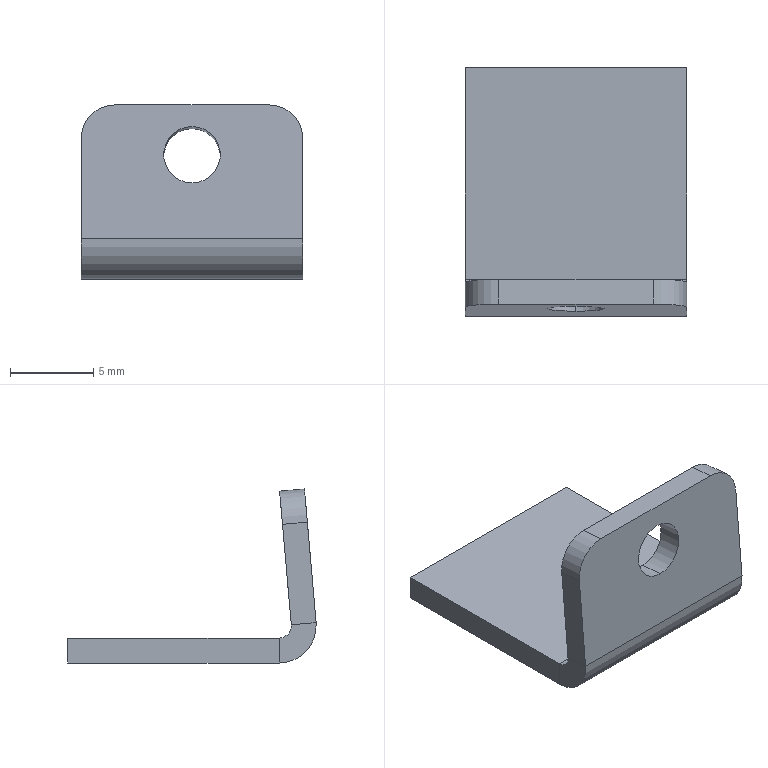Part | STEP file | 07-10 reflector plate (Default) | 1 solid | 18 faces | box 13.3 x 14.933 x 10.46 mm | volume 447.05 mm3 | plane 12 | cylinder 6 | commonest cylinder face diameters 3.4 x2 4 x2 1.473 x1 4.473 x1
STEP:
#1=CARTESIAN_POINT('',(0.,-7.585,7.665));
#2=VERTEX_POINT('',#1);
#3=CARTESIAN_POINT('',(0.,-7.881,4.278));
#4=VERTEX_POINT('',#3);
#5=CARTESIAN_POINT('',(0.,-7.733,5.971));
#6=DIRECTION('',(0.,-0.9962,0.08716));
#7=DIRECTION('',(0.,-0.08716,-0.9962));
#8=AXIS2_PLACEMENT_3D('',#5,#6,#7);
#9=CIRCLE('',#8,1.7);
#10=EDGE_CURVE('',#2,#4,#9,.T.);
#11=ORIENTED_EDGE('',*,*,#10,.T.);
#12=CARTESIAN_POINT('',(0.,-6.387,4.147));
#13=VERTEX_POINT('',#12);
#14=CARTESIAN_POINT('',(0.,-16.349,5.019));
#15=DIRECTION('',(0.,0.9962,-0.08716));
#16=VECTOR('',#15,1000.);
#17=LINE('',#14,#16);
#18=EDGE_CURVE('',#4,#13,#17,.T.);
#19=ORIENTED_EDGE('',*,*,#18,.T.);
#20=CARTESIAN_POINT('',(0.,-6.091,7.534));
#21=VERTEX_POINT('',#20);
#22=CARTESIAN_POINT('',(0.,-6.239,5.841));
#23=DIRECTION('',(0.,0.9962,-0.08716));
#24=DIRECTION('',(0.,0.08716,0.9962));
#25=AXIS2_PLACEMENT_3D('',#22,#23,#24);
#26=CIRCLE('',#25,1.7);
#27=EDGE_CURVE('',#13,#21,#26,.T.);
#28=ORIENTED_EDGE('',*,*,#27,.T.);
#29=CARTESIAN_POINT('',(0.,-16.053,8.406));
#30=DIRECTION('',(0.,0.9962,-0.08716));
#31=VECTOR('',#30,1000.);
#32=LINE('',#29,#31);
#33=EDGE_CURVE('',#2,#21,#32,.T.);
#34=ORIENTED_EDGE('',*,*,#33,.F.);
#35=EDGE_LOOP('',(#11,#19,#28,#34));
#36=FACE_OUTER_BOUND('',#35,.T.);
#37=CARTESIAN_POINT('',(0.,-16.201,6.712));
#38=DIRECTION('',(0.,0.9962,-0.08716));
#39=DIRECTION('',(0.,0.08716,0.9962));
#40=AXIS2_PLACEMENT_3D('',#37,#38,#39);
#41=CYLINDRICAL_SURFACE('',#40,1.7);
#42=ADVANCED_FACE('',(#36),#41,.F.);
#43=CARTESIAN_POINT('',(6.65,-5.946,0.));
#44=VERTEX_POINT('',#43);
#45=CARTESIAN_POINT('',(6.65,6.75,0.));
#46=VERTEX_POINT('',#45);
#47=CARTESIAN_POINT('',(6.65,6.75,0.));
#48=DIRECTION('',(0.,1.,0.));
#49=VECTOR('',#48,1000.);
#50=LINE('',#47,#49);
#51=EDGE_CURVE('',#44,#46,#50,.T.);
#52=ORIENTED_EDGE('',*,*,#51,.F.);
#53=CARTESIAN_POINT('',(6.65,-5.946,-1.5));
#54=VERTEX_POINT('',#53);
#55=CARTESIAN_POINT('',(6.65,-5.946,0.));
#56=DIRECTION('',(0.,0.,-1.));
#57=VECTOR('',#56,1000.);
#58=LINE('',#55,#57);
#59=EDGE_CURVE('',#44,#54,#58,.T.);
#60=ORIENTED_EDGE('',*,*,#59,.T.);
#61=CARTESIAN_POINT('',(6.65,6.75,-1.5));
#62=VERTEX_POINT('',#61);
#63=CARTESIAN_POINT('',(6.65,6.75,-1.5));
#64=DIRECTION('',(0.,1.,0.));
#65=VECTOR('',#64,1000.);
#66=LINE('',#63,#65);
#67=EDGE_CURVE('',#54,#62,#66,.T.);
#68=ORIENTED_EDGE('',*,*,#67,.T.);
#69=CARTESIAN_POINT('',(6.65,6.75,-1.5));
#70=DIRECTION('',(0.,0.,1.));
#71=VECTOR('',#70,1000.);
#72=LINE('',#69,#71);
#73=EDGE_CURVE('',#62,#46,#72,.T.);
#74=ORIENTED_EDGE('',*,*,#73,.T.);
#75=EDGE_LOOP('',(#52,#60,#68,#74));
#76=FACE_OUTER_BOUND('',#75,.T.);
#77=CARTESIAN_POINT('',(6.65,6.75,-1.5));
#78=DIRECTION('',(1.,0.,0.));
#79=DIRECTION('',(0.,1.,0.));
#80=AXIS2_PLACEMENT_3D('',#77,#78,#79);
#81=PLANE('',#80);
#82=ADVANCED_FACE('',(#76),#81,.T.);
#83=CARTESIAN_POINT('',(-6.65,-5.946,-1.5));
#84=VERTEX_POINT('',#83);
#85=CARTESIAN_POINT('',(6.65,-5.946,-1.5));
#86=DIRECTION('',(-1.,0.,0.));
#87=VECTOR('',#86,1000.);
#88=LINE('',#85,#87);
#89=EDGE_CURVE('',#54,#84,#88,.T.);
#90=ORIENTED_EDGE('',*,*,#89,.T.);
#91=CARTESIAN_POINT('',(-6.65,6.75,-1.5));
#92=VERTEX_POINT('',#91);
#93=CARTESIAN_POINT('',(-6.65,6.75,-1.5));
#94=DIRECTION('',(0.,-1.,0.));
#95=VECTOR('',#94,1000.);
#96=LINE('',#93,#95);
#97=EDGE_CURVE('',#92,#84,#96,.T.);
#98=ORIENTED_EDGE('',*,*,#97,.F.);
#99=CARTESIAN_POINT('',(-6.65,6.75,-1.5));
#100=DIRECTION('',(-1.,0.,0.));
#101=VECTOR('',#100,1000.);
#102=LINE('',#99,#101);
#103=EDGE_CURVE('',#62,#92,#102,.T.);
#104=ORIENTED_EDGE('',*,*,#103,.F.);
#105=ORIENTED_EDGE('',*,*,#67,.F.);
#106=EDGE_LOOP('',(#90,#98,#104,#105));
#107=FACE_OUTER_BOUND('',#106,.T.);
#108=CARTESIAN_POINT('',(6.65,-6.75,-1.5));
#109=DIRECTION('',(0.,0.,1.));
#110=DIRECTION('',(1.,0.,0.));
#111=AXIS2_PLACEMENT_3D('',#108,#109,#110);
#112=PLANE('',#111);
#113=ADVANCED_FACE('',(#107),#112,.F.);
#114=CARTESIAN_POINT('',(-6.65,6.75,0.));
#115=VERTEX_POINT('',#114);
#116=CARTESIAN_POINT('',(-6.65,-5.946,0.));
#117=VERTEX_POINT('',#116);
#118=CARTESIAN_POINT('',(-6.65,6.75,0.));
#119=DIRECTION('',(0.,-1.,0.));
#120=VECTOR('',#119,1000.);
#121=LINE('',#118,#120);
#122=EDGE_CURVE('',#115,#117,#121,.T.);
#123=ORIENTED_EDGE('',*,*,#122,.T.);
#124=CARTESIAN_POINT('',(6.65,-5.946,0.));
#125=DIRECTION('',(-1.,0.,0.));
#126=VECTOR('',#125,1000.);
#127=LINE('',#124,#126);
#128=EDGE_CURVE('',#44,#117,#127,.T.);
#129=ORIENTED_EDGE('',*,*,#128,.F.);
#130=ORIENTED_EDGE('',*,*,#51,.T.);
#131=CARTESIAN_POINT('',(-6.65,6.75,0.));
#132=DIRECTION('',(-1.,0.,0.));
#133=VECTOR('',#132,1000.);
#134=LINE('',#131,#133);
#135=EDGE_CURVE('',#46,#115,#134,.T.);
#136=ORIENTED_EDGE('',*,*,#135,.T.);
#137=EDGE_LOOP('',(#123,#129,#130,#136));
#138=FACE_OUTER_BOUND('',#137,.T.);
#139=CARTESIAN_POINT('',(6.65,-6.75,0.));
#140=DIRECTION('',(0.,0.,1.));
#141=DIRECTION('',(1.,0.,0.));
#142=AXIS2_PLACEMENT_3D('',#139,#140,#141);
#143=PLANE('',#142);
#144=ADVANCED_FACE('',(#138),#143,.T.);
#145=CARTESIAN_POINT('',(-6.65,-5.946,0.));
#146=DIRECTION('',(0.,0.,-1.));
#147=VECTOR('',#146,1000.);
#148=LINE('',#145,#147);
#149=EDGE_CURVE('',#117,#84,#148,.T.);
#150=ORIENTED_EDGE('',*,*,#149,.F.);
#151=ORIENTED_EDGE('',*,*,#122,.F.);
#152=CARTESIAN_POINT('',(-6.65,6.75,-1.5));
#153=DIRECTION('',(0.,0.,1.));
#154=VECTOR('',#153,1000.);
#155=LINE('',#152,#154);
#156=EDGE_CURVE('',#92,#115,#155,.T.);
#157=ORIENTED_EDGE('',*,*,#156,.F.);
#158=ORIENTED_EDGE('',*,*,#97,.T.);
#159=EDGE_LOOP('',(#150,#151,#157,#158));
#160=FACE_OUTER_BOUND('',#159,.T.);
#161=CARTESIAN_POINT('',(-6.65,6.75,-1.5));
#162=DIRECTION('',(-1.,0.,0.));
#163=DIRECTION('',(0.,-1.,0.));
#164=AXIS2_PLACEMENT_3D('',#161,#162,#163);
#165=PLANE('',#164);
#166=ADVANCED_FACE('',(#160),#165,.T.);
#167=ORIENTED_EDGE('',*,*,#135,.F.);
#168=ORIENTED_EDGE('',*,*,#73,.F.);
#169=ORIENTED_EDGE('',*,*,#103,.T.);
#170=ORIENTED_EDGE('',*,*,#156,.T.);
#171=EDGE_LOOP('',(#167,#168,#169,#170));
#172=FACE_OUTER_BOUND('',#171,.T.);
#173=CARTESIAN_POINT('',(-6.65,6.75,-1.5));
#174=DIRECTION('',(0.,1.,0.));
#175=DIRECTION('',(0.,0.,1.));
#176=AXIS2_PLACEMENT_3D('',#173,#174,#175);
#177=PLANE('',#176);
#178=ADVANCED_FACE('',(#172),#177,.T.);
#179=CARTESIAN_POINT('',(-6.65,-6.68,0.8008));
#180=VERTEX_POINT('',#179);
#181=CARTESIAN_POINT('',(-6.65,-8.174,0.9315));
#182=VERTEX_POINT('',#181);
#183=CARTESIAN_POINT('',(-6.65,-6.68,0.8008));
#184=DIRECTION('',(0.,-0.9962,0.08716));
#185=VECTOR('',#184,1000.);
#186=LINE('',#183,#185);
#187=EDGE_CURVE('',#180,#182,#186,.T.);
#188=ORIENTED_EDGE('',*,*,#187,.F.);
#189=CARTESIAN_POINT('',(-6.65,-5.946,0.7366));
#190=DIRECTION('',(-1.,0.,0.));
#191=DIRECTION('',(0.,0.,-1.));
#192=AXIS2_PLACEMENT_3D('',#189,#190,#191);
#193=CIRCLE('',#192,0.7366);
#194=EDGE_CURVE('',#117,#180,#193,.T.);
#195=ORIENTED_EDGE('',*,*,#194,.F.);
#196=ORIENTED_EDGE('',*,*,#149,.T.);
#197=CARTESIAN_POINT('',(-6.65,-5.946,0.7366));
#198=DIRECTION('',(-1.,0.,0.));
#199=DIRECTION('',(0.,0.,-1.));
#200=AXIS2_PLACEMENT_3D('',#197,#198,#199);
#201=CIRCLE('',#200,2.237);
#202=EDGE_CURVE('',#84,#182,#201,.T.);
#203=ORIENTED_EDGE('',*,*,#202,.T.);
#204=EDGE_LOOP('',(#188,#195,#196,#203));
#205=FACE_OUTER_BOUND('',#204,.T.);
#206=CARTESIAN_POINT('',(-6.65,-5.946,0.7366));
#207=DIRECTION('',(-1.,0.,0.));
#208=DIRECTION('',(0.,0.,1.));
#209=AXIS2_PLACEMENT_3D('',#206,#207,#208);
#210=PLANE('',#209);
#211=ADVANCED_FACE('',(#205),#210,.T.);
#212=CARTESIAN_POINT('',(6.65,-6.68,0.8008));
#213=VERTEX_POINT('',#212);
#214=CARTESIAN_POINT('',(6.65,-5.946,0.7366));
#215=DIRECTION('',(1.,0.,0.));
#216=DIRECTION('',(0.,0.,-1.));
#217=AXIS2_PLACEMENT_3D('',#214,#215,#216);
#218=CIRCLE('',#217,0.7366);
#219=EDGE_CURVE('',#213,#44,#218,.T.);
#220=ORIENTED_EDGE('',*,*,#219,.F.);
#221=CARTESIAN_POINT('',(6.65,-8.174,0.9315));
#222=VERTEX_POINT('',#221);
#223=CARTESIAN_POINT('',(6.65,-6.68,0.8008));
#224=DIRECTION('',(0.,-0.9962,0.08716));
#225=VECTOR('',#224,1000.);
#226=LINE('',#223,#225);
#227=EDGE_CURVE('',#213,#222,#226,.T.);
#228=ORIENTED_EDGE('',*,*,#227,.T.);
#229=CARTESIAN_POINT('',(6.65,-5.946,0.7366));
#230=DIRECTION('',(1.,0.,0.));
#231=DIRECTION('',(0.,0.,-1.));
#232=AXIS2_PLACEMENT_3D('',#229,#230,#231);
#233=CIRCLE('',#232,2.237);
#234=EDGE_CURVE('',#222,#54,#233,.T.);
#235=ORIENTED_EDGE('',*,*,#234,.T.);
#236=ORIENTED_EDGE('',*,*,#59,.F.);
#237=EDGE_LOOP('',(#220,#228,#235,#236));
#238=FACE_OUTER_BOUND('',#237,.T.);
#239=CARTESIAN_POINT('',(6.65,-5.946,0.7366));
#240=DIRECTION('',(-1.,0.,0.));
#241=DIRECTION('',(0.,0.,1.));
#242=AXIS2_PLACEMENT_3D('',#239,#240,#241);
#243=PLANE('',#242);
#244=ADVANCED_FACE('',(#238),#243,.F.);
#245=ORIENTED_EDGE('',*,*,#89,.F.);
#246=ORIENTED_EDGE('',*,*,#234,.F.);
#247=CARTESIAN_POINT('',(6.65,-8.174,0.9315));
#248=DIRECTION('',(1.,0.,0.));
#249=VECTOR('',#248,1000.);
#250=LINE('',#247,#249);
#251=EDGE_CURVE('',#182,#222,#250,.T.);
#252=ORIENTED_EDGE('',*,*,#251,.F.);
#253=ORIENTED_EDGE('',*,*,#202,.F.);
#254=EDGE_LOOP('',(#245,#246,#252,#253));
#255=FACE_OUTER_BOUND('',#254,.T.);
#256=CARTESIAN_POINT('',(6.65,-5.946,0.7366));
#257=DIRECTION('',(1.,0.,0.));
#258=DIRECTION('',(0.,-0.9962,0.08716));
#259=AXIS2_PLACEMENT_3D('',#256,#257,#258);
#260=CYLINDRICAL_SURFACE('',#259,2.237);
#261=ADVANCED_FACE('',(#255),#260,.T.);
#262=ORIENTED_EDGE('',*,*,#128,.T.);
#263=ORIENTED_EDGE('',*,*,#194,.T.);
#264=CARTESIAN_POINT('',(-6.65,-6.68,0.8008));
#265=DIRECTION('',(1.,0.,0.));
#266=VECTOR('',#265,1000.);
#267=LINE('',#264,#266);
#268=EDGE_CURVE('',#180,#213,#267,.T.);
#269=ORIENTED_EDGE('',*,*,#268,.T.);
#270=ORIENTED_EDGE('',*,*,#219,.T.);
#271=EDGE_LOOP('',(#262,#263,#269,#270));
#272=FACE_OUTER_BOUND('',#271,.T.);
#273=CARTESIAN_POINT('',(6.65,-5.946,0.7366));
#274=DIRECTION('',(1.,0.,0.));
#275=DIRECTION('',(0.,-0.9962,0.08716));
#276=AXIS2_PLACEMENT_3D('',#273,#274,#275);
#277=CYLINDRICAL_SURFACE('',#276,0.7366);
#278=ADVANCED_FACE('',(#272),#277,.F.);
#279=CARTESIAN_POINT('',(6.65,-6.152,6.837));
#280=VERTEX_POINT('',#279);
#281=CARTESIAN_POINT('',(6.65,-6.75,0.));
#282=DIRECTION('',(0.,-0.08716,-0.9962));
#283=VECTOR('',#282,1000.);
#284=LINE('',#281,#283);
#285=EDGE_CURVE('',#280,#213,#284,.T.);
#286=ORIENTED_EDGE('',*,*,#285,.F.);
#287=CARTESIAN_POINT('',(6.65,-7.646,6.968));
#288=VERTEX_POINT('',#287);
#289=CARTESIAN_POINT('',(6.65,-7.646,6.968));
#290=DIRECTION('',(0.,-0.9962,0.08716));
#291=VECTOR('',#290,1000.);
#292=LINE('',#289,#291);
#293=EDGE_CURVE('',#280,#288,#292,.T.);
#294=ORIENTED_EDGE('',*,*,#293,.T.);
#295=CARTESIAN_POINT('',(6.65,-8.244,0.1307));
#296=DIRECTION('',(0.,-0.08716,-0.9962));
#297=VECTOR('',#296,1000.);
#298=LINE('',#295,#297);
#299=EDGE_CURVE('',#288,#222,#298,.T.);
#300=ORIENTED_EDGE('',*,*,#299,.T.);
#301=ORIENTED_EDGE('',*,*,#227,.F.);
#302=EDGE_LOOP('',(#286,#294,#300,#301));
#303=FACE_OUTER_BOUND('',#302,.T.);
#304=CARTESIAN_POINT('',(6.65,-8.244,0.1307));
#305=DIRECTION('',(1.,0.,0.));
#306=DIRECTION('',(0.,0.,-1.));
#307=AXIS2_PLACEMENT_3D('',#304,#305,#306);
#308=PLANE('',#307);
#309=ADVANCED_FACE('',(#303),#308,.T.);
#310=CARTESIAN_POINT('',(-6.65,-7.646,6.968));
#311=VERTEX_POINT('',#310);
#312=CARTESIAN_POINT('',(-6.65,-7.472,8.96));
#313=DIRECTION('',(0.,0.08716,0.9962));
#314=VECTOR('',#313,1000.);
#315=LINE('',#312,#314);
#316=EDGE_CURVE('',#182,#311,#315,.T.);
#317=ORIENTED_EDGE('',*,*,#316,.T.);
#318=CARTESIAN_POINT('',(-6.65,-6.152,6.837));
#319=VERTEX_POINT('',#318);
#320=CARTESIAN_POINT('',(-6.65,-7.646,6.968));
#321=DIRECTION('',(0.,0.9962,-0.08716));
#322=VECTOR('',#321,1000.);
#323=LINE('',#320,#322);
#324=EDGE_CURVE('',#311,#319,#323,.T.);
#325=ORIENTED_EDGE('',*,*,#324,.T.);
#326=CARTESIAN_POINT('',(-6.65,-5.978,8.829));
#327=DIRECTION('',(0.,0.08716,0.9962));
#328=VECTOR('',#327,1000.);
#329=LINE('',#326,#328);
#330=EDGE_CURVE('',#180,#319,#329,.T.);
#331=ORIENTED_EDGE('',*,*,#330,.F.);
#332=ORIENTED_EDGE('',*,*,#187,.T.);
#333=EDGE_LOOP('',(#317,#325,#331,#332));
#334=FACE_OUTER_BOUND('',#333,.T.);
#335=CARTESIAN_POINT('',(-6.65,-7.472,8.96));
#336=DIRECTION('',(-1.,0.,0.));
#337=DIRECTION('',(0.,0.,1.));
#338=AXIS2_PLACEMENT_3D('',#335,#336,#337);
#339=PLANE('',#338);
#340=ADVANCED_FACE('',(#334),#339,.T.);
#341=ORIENTED_EDGE('',*,*,#10,.F.);
#342=CARTESIAN_POINT('',(0.,-7.733,5.971));
#343=DIRECTION('',(0.,-0.9962,0.08716));
#344=DIRECTION('',(0.,-0.08716,-0.9962));
#345=AXIS2_PLACEMENT_3D('',#342,#343,#344);
#346=CIRCLE('',#345,1.7);
#347=EDGE_CURVE('',#4,#2,#346,.T.);
#348=ORIENTED_EDGE('',*,*,#347,.F.);
#349=EDGE_LOOP('',(#341,#348));
#350=FACE_BOUND('',#349,.T.);
#351=ORIENTED_EDGE('',*,*,#299,.F.);
#352=CARTESIAN_POINT('',(4.65,-7.472,8.96));
#353=VERTEX_POINT('',#352);
#354=CARTESIAN_POINT('',(4.65,-7.646,6.968));
#355=DIRECTION('',(0.,-0.9962,0.08716));
#356=DIRECTION('',(0.,-0.08716,-0.9962));
#357=AXIS2_PLACEMENT_3D('',#354,#355,#356);
#358=CIRCLE('',#357,2.);
#359=EDGE_CURVE('',#288,#353,#358,.T.);
#360=ORIENTED_EDGE('',*,*,#359,.T.);
#361=CARTESIAN_POINT('',(-4.65,-7.472,8.96));
#362=VERTEX_POINT('',#361);
#363=CARTESIAN_POINT('',(6.65,-7.472,8.96));
#364=DIRECTION('',(1.,0.,0.));
#365=VECTOR('',#364,1000.);
#366=LINE('',#363,#365);
#367=EDGE_CURVE('',#362,#353,#366,.T.);
#368=ORIENTED_EDGE('',*,*,#367,.F.);
#369=CARTESIAN_POINT('',(-4.65,-7.646,6.968));
#370=DIRECTION('',(0.,-0.9962,0.08716));
#371=DIRECTION('',(0.,-0.08716,-0.9962));
#372=AXIS2_PLACEMENT_3D('',#369,#370,#371);
#373=CIRCLE('',#372,2.);
#374=EDGE_CURVE('',#362,#311,#373,.T.);
#375=ORIENTED_EDGE('',*,*,#374,.T.);
#376=ORIENTED_EDGE('',*,*,#316,.F.);
#377=ORIENTED_EDGE('',*,*,#251,.T.);
#378=EDGE_LOOP('',(#351,#360,#368,#375,#376,#377));
#379=FACE_OUTER_BOUND('',#378,.T.);
#380=CARTESIAN_POINT('',(6.65,-8.244,0.1307));
#381=DIRECTION('',(0.,-0.9962,0.08716));
#382=DIRECTION('',(0.,-0.08716,-0.9962));
#383=AXIS2_PLACEMENT_3D('',#380,#381,#382);
#384=PLANE('',#383);
#385=ADVANCED_FACE('',(#350,#379),#384,.T.);
#386=CARTESIAN_POINT('',(0.,-6.239,5.841));
#387=DIRECTION('',(0.,0.9962,-0.08716));
#388=DIRECTION('',(0.,0.08716,0.9962));
#389=AXIS2_PLACEMENT_3D('',#386,#387,#388);
#390=CIRCLE('',#389,1.7);
#391=EDGE_CURVE('',#21,#13,#390,.T.);
#392=ORIENTED_EDGE('',*,*,#391,.F.);
#393=ORIENTED_EDGE('',*,*,#27,.F.);
#394=EDGE_LOOP('',(#392,#393));
#395=FACE_BOUND('',#394,.T.);
#396=CARTESIAN_POINT('',(-4.65,-5.978,8.829));
#397=VERTEX_POINT('',#396);
#398=CARTESIAN_POINT('',(4.65,-5.978,8.829));
#399=VERTEX_POINT('',#398);
#400=CARTESIAN_POINT('',(6.65,-5.978,8.829));
#401=DIRECTION('',(1.,0.,0.));
#402=VECTOR('',#401,1000.);
#403=LINE('',#400,#402);
#404=EDGE_CURVE('',#397,#399,#403,.T.);
#405=ORIENTED_EDGE('',*,*,#404,.T.);
#406=CARTESIAN_POINT('',(4.65,-6.152,6.837));
#407=DIRECTION('',(0.,0.9962,-0.08716));
#408=DIRECTION('',(0.,-0.08716,-0.9962));
#409=AXIS2_PLACEMENT_3D('',#406,#407,#408);
#410=CIRCLE('',#409,2.);
#411=EDGE_CURVE('',#399,#280,#410,.T.);
#412=ORIENTED_EDGE('',*,*,#411,.T.);
#413=ORIENTED_EDGE('',*,*,#285,.T.);
#414=ORIENTED_EDGE('',*,*,#268,.F.);
#415=ORIENTED_EDGE('',*,*,#330,.T.);
#416=CARTESIAN_POINT('',(-4.65,-6.152,6.837));
#417=DIRECTION('',(0.,0.9962,-0.08716));
#418=DIRECTION('',(0.,-0.08716,-0.9962));
#419=AXIS2_PLACEMENT_3D('',#416,#417,#418);
#420=CIRCLE('',#419,2.);
#421=EDGE_CURVE('',#319,#397,#420,.T.);
#422=ORIENTED_EDGE('',*,*,#421,.T.);
#423=EDGE_LOOP('',(#405,#412,#413,#414,#415,#422));
#424=FACE_OUTER_BOUND('',#423,.T.);
#425=CARTESIAN_POINT('',(6.65,-6.75,0.));
#426=DIRECTION('',(0.,-0.9962,0.08716));
#427=DIRECTION('',(0.,-0.08716,-0.9962));
#428=AXIS2_PLACEMENT_3D('',#425,#426,#427);
#429=PLANE('',#428);
#430=ADVANCED_FACE('',(#395,#424),#429,.F.);
#431=ORIENTED_EDGE('',*,*,#367,.T.);
#432=CARTESIAN_POINT('',(4.65,-7.472,8.96));
#433=DIRECTION('',(0.,0.9962,-0.08716));
#434=VECTOR('',#433,1000.);
#435=LINE('',#432,#434);
#436=EDGE_CURVE('',#353,#399,#435,.T.);
#437=ORIENTED_EDGE('',*,*,#436,.T.);
#438=ORIENTED_EDGE('',*,*,#404,.F.);
#439=CARTESIAN_POINT('',(-4.65,-7.472,8.96));
#440=DIRECTION('',(0.,-0.9962,0.08716));
#441=VECTOR('',#440,1000.);
#442=LINE('',#439,#441);
#443=EDGE_CURVE('',#397,#362,#442,.T.);
#444=ORIENTED_EDGE('',*,*,#443,.T.);
#445=EDGE_LOOP('',(#431,#437,#438,#444));
#446=FACE_OUTER_BOUND('',#445,.T.);
#447=CARTESIAN_POINT('',(6.65,-7.472,8.96));
#448=DIRECTION('',(0.,0.08716,0.9962));
#449=DIRECTION('',(0.,-0.9962,0.08716));
#450=AXIS2_PLACEMENT_3D('',#447,#448,#449);
#451=PLANE('',#450);
#452=ADVANCED_FACE('',(#446),#451,.T.);
#453=ORIENTED_EDGE('',*,*,#359,.F.);
#454=ORIENTED_EDGE('',*,*,#293,.F.);
#455=ORIENTED_EDGE('',*,*,#411,.F.);
#456=ORIENTED_EDGE('',*,*,#436,.F.);
#457=EDGE_LOOP('',(#453,#454,#455,#456));
#458=FACE_OUTER_BOUND('',#457,.T.);
#459=CARTESIAN_POINT('',(4.65,-7.646,6.968));
#460=DIRECTION('',(0.,0.9962,-0.08716));
#461=DIRECTION('',(0.,0.08716,0.9962));
#462=AXIS2_PLACEMENT_3D('',#459,#460,#461);
#463=CYLINDRICAL_SURFACE('',#462,2.);
#464=ADVANCED_FACE('',(#458),#463,.T.);
#465=ORIENTED_EDGE('',*,*,#374,.F.);
#466=ORIENTED_EDGE('',*,*,#443,.F.);
#467=ORIENTED_EDGE('',*,*,#421,.F.);
#468=ORIENTED_EDGE('',*,*,#324,.F.);
#469=EDGE_LOOP('',(#465,#466,#467,#468));
#470=FACE_OUTER_BOUND('',#469,.T.);
#471=CARTESIAN_POINT('',(-4.65,-7.646,6.968));
#472=DIRECTION('',(0.,0.9962,-0.08716));
#473=DIRECTION('',(0.,0.08716,0.9962));
#474=AXIS2_PLACEMENT_3D('',#471,#472,#473);
#475=CYLINDRICAL_SURFACE('',#474,2.);
#476=ADVANCED_FACE('',(#470),#475,.T.);
#477=ORIENTED_EDGE('',*,*,#18,.F.);
#478=ORIENTED_EDGE('',*,*,#347,.T.);
#479=ORIENTED_EDGE('',*,*,#33,.T.);
#480=ORIENTED_EDGE('',*,*,#391,.T.);
#481=EDGE_LOOP('',(#477,#478,#479,#480));
#482=FACE_OUTER_BOUND('',#481,.T.);
#483=CARTESIAN_POINT('',(0.,-16.201,6.712));
#484=DIRECTION('',(0.,0.9962,-0.08716));
#485=DIRECTION('',(0.,0.08716,0.9962));
#486=AXIS2_PLACEMENT_3D('',#483,#484,#485);
#487=CYLINDRICAL_SURFACE('',#486,1.7);
#488=ADVANCED_FACE('',(#482),#487,.F.);
#489=CLOSED_SHELL('',(#42,#82,#113,#144,#166,#178,#211,#244,#261,#278,#309,#340,#385,#430,#452,#464,#476,#488));
#490=MANIFOLD_SOLID_BREP('',#489);
#491=CARTESIAN_POINT('',(0.,0.,0.));
#492=DIRECTION('',(0.,0.,1.));
#493=DIRECTION('',(1.,0.,0.));
#494=AXIS2_PLACEMENT_3D('',#491,#492,#493);
#495=(LENGTH_UNIT()NAMED_UNIT(*)SI_UNIT(.MILLI.,.METRE.));
#496=UNCERTAINTY_MEASURE_WITH_UNIT(LENGTH_MEASURE(0.00001),#495,'','');
#497=(NAMED_UNIT(*)PLANE_ANGLE_UNIT()SI_UNIT($,.RADIAN.));
#498=(NAMED_UNIT(*)SI_UNIT($,.STERADIAN.)SOLID_ANGLE_UNIT());
#499=(GEOMETRIC_REPRESENTATION_CONTEXT(3)GLOBAL_UNCERTAINTY_ASSIGNED_CONTEXT((#496))GLOBAL_UNIT_ASSIGNED_CONTEXT((#495,#497,#498))REPRESENTATION_CONTEXT('',''));
#500=ADVANCED_BREP_SHAPE_REPRESENTATION('',(#490,#494),#499);